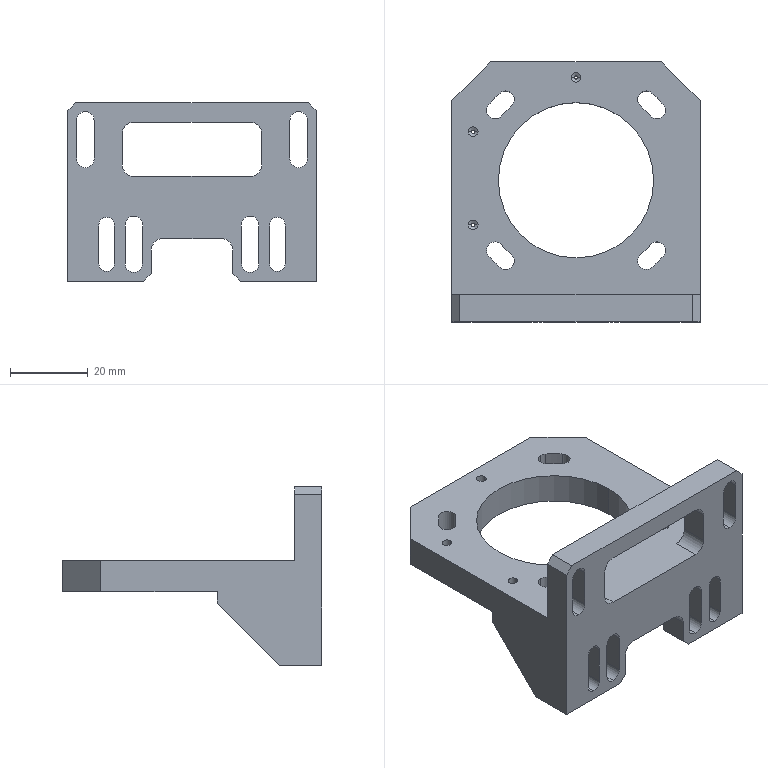Part | 1 solid | 101 faces | box 64 x 67 x 46 mm | volume 33860 mm3 | cylinder 54 | plane 41 | cone 6 | commonest cylinder face diameters 4.4 x12 4.5 x12 6 x8 2.5 x6 4 x6 50.75 x4